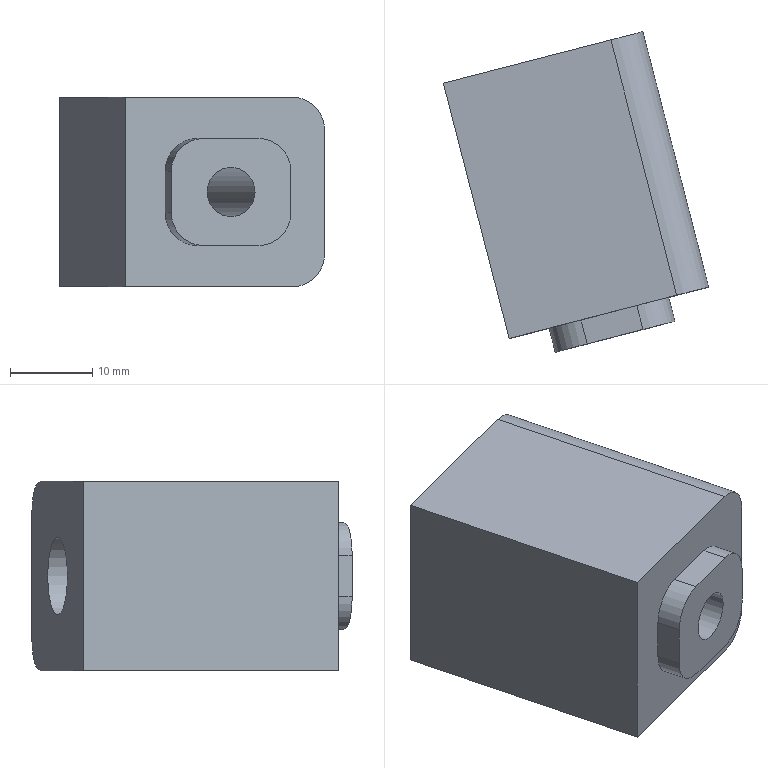Part | STEP file | 车灯-后视镜_id46_x_t | 1 solid | 20 faces | box 32.198 x 38.885 x 23 mm | volume 17479 mm3 | plane 12 | cylinder 8 | commonest cylinder face diameters 8 x6 6 x1 9.5 x1
STEP:
#1=CARTESIAN_POINT('',(-81.034,92.171,88.714));
#2=VERTEX_POINT('',#1);
#3=CARTESIAN_POINT('',(-81.034,92.171,103.714));
#4=VERTEX_POINT('',#3);
#5=CARTESIAN_POINT('',(-81.034,92.171,96.214));
#6=DIRECTION('',(0.,0.,1.));
#7=VECTOR('',#6,1.);
#8=LINE('',#5,#7);
#9=EDGE_CURVE('',#2,#4,#8,.T.);
#10=ORIENTED_EDGE('',*,*,#9,.T.);
#11=CARTESIAN_POINT('',(-84.907,91.172,107.714));
#12=VERTEX_POINT('',#11);
#13=CARTESIAN_POINT('',(-84.907,91.172,103.714));
#14=DIRECTION('',(0.2497,-0.9683,0.));
#15=DIRECTION('',(0.9683,0.2497,0.));
#16=AXIS2_PLACEMENT_3D('',#13,#14,#15);
#17=CIRCLE('',#16,4.);
#18=EDGE_CURVE('',#4,#12,#17,.T.);
#19=ORIENTED_EDGE('',*,*,#18,.T.);
#20=CARTESIAN_POINT('',(-105.242,85.928,107.714));
#21=VERTEX_POINT('',#20);
#22=CARTESIAN_POINT('',(-79.081,92.674,107.714));
#23=DIRECTION('',(-0.9683,-0.2497,0.));
#24=VECTOR('',#23,1.);
#25=LINE('',#22,#24);
#26=EDGE_CURVE('',#12,#21,#25,.T.);
#27=ORIENTED_EDGE('',*,*,#26,.T.);
#28=CARTESIAN_POINT('',(-105.242,85.928,84.714));
#29=VERTEX_POINT('',#28);
#30=CARTESIAN_POINT('',(-105.242,85.928,96.214));
#31=DIRECTION('',(0.,0.,1.));
#32=VECTOR('',#31,1.);
#33=LINE('',#30,#32);
#34=EDGE_CURVE('',#29,#21,#33,.T.);
#35=ORIENTED_EDGE('',*,*,#34,.F.);
#36=CARTESIAN_POINT('',(-84.907,91.172,84.714));
#37=VERTEX_POINT('',#36);
#38=CARTESIAN_POINT('',(-79.081,92.674,84.714));
#39=DIRECTION('',(0.9683,0.2497,0.));
#40=VECTOR('',#39,1.);
#41=LINE('',#38,#40);
#42=EDGE_CURVE('',#29,#37,#41,.T.);
#43=ORIENTED_EDGE('',*,*,#42,.T.);
#44=CARTESIAN_POINT('',(-84.907,91.172,88.714));
#45=DIRECTION('',(0.2497,-0.9683,0.));
#46=DIRECTION('',(0.9683,0.2497,0.));
#47=AXIS2_PLACEMENT_3D('',#44,#45,#46);
#48=CIRCLE('',#47,4.);
#49=EDGE_CURVE('',#37,#2,#48,.T.);
#50=ORIENTED_EDGE('',*,*,#49,.T.);
#51=EDGE_LOOP('',(#10,#19,#27,#35,#43,#50));
#52=FACE_BOUND('',#51,.T.);
#53=CARTESIAN_POINT('',(-89.749,89.923,89.714));
#54=VERTEX_POINT('',#53);
#55=CARTESIAN_POINT('',(-96.527,88.175,89.714));
#56=VERTEX_POINT('',#55);
#57=CARTESIAN_POINT('',(-105.242,85.928,89.714));
#58=DIRECTION('',(-0.9683,-0.2497,0.));
#59=VECTOR('',#58,1.);
#60=LINE('',#57,#59);
#61=EDGE_CURVE('',#54,#56,#60,.T.);
#62=ORIENTED_EDGE('',*,*,#61,.T.);
#63=CARTESIAN_POINT('',(-100.4,87.177,93.714));
#64=VERTEX_POINT('',#63);
#65=CARTESIAN_POINT('',(-96.527,88.175,93.714));
#66=DIRECTION('',(-0.2497,0.9683,0.));
#67=DIRECTION('',(0.9683,0.2497,0.));
#68=AXIS2_PLACEMENT_3D('',#65,#66,#67);
#69=CIRCLE('',#68,4.);
#70=EDGE_CURVE('',#56,#64,#69,.T.);
#71=ORIENTED_EDGE('',*,*,#70,.T.);
#72=CARTESIAN_POINT('',(-100.4,87.177,98.714));
#73=VERTEX_POINT('',#72);
#74=CARTESIAN_POINT('',(-100.4,87.177,107.714));
#75=DIRECTION('',(0.,0.,1.));
#76=VECTOR('',#75,1.);
#77=LINE('',#74,#76);
#78=EDGE_CURVE('',#64,#73,#77,.T.);
#79=ORIENTED_EDGE('',*,*,#78,.T.);
#80=CARTESIAN_POINT('',(-96.527,88.175,102.714));
#81=VERTEX_POINT('',#80);
#82=CARTESIAN_POINT('',(-96.527,88.175,98.714));
#83=DIRECTION('',(-0.2497,0.9683,0.));
#84=DIRECTION('',(0.9683,0.2497,0.));
#85=AXIS2_PLACEMENT_3D('',#82,#83,#84);
#86=CIRCLE('',#85,4.);
#87=EDGE_CURVE('',#73,#81,#86,.T.);
#88=ORIENTED_EDGE('',*,*,#87,.T.);
#89=CARTESIAN_POINT('',(-89.749,89.923,102.714));
#90=VERTEX_POINT('',#89);
#91=CARTESIAN_POINT('',(-105.242,85.928,102.714));
#92=DIRECTION('',(0.9683,0.2497,0.));
#93=VECTOR('',#92,1.);
#94=LINE('',#91,#93);
#95=EDGE_CURVE('',#81,#90,#94,.T.);
#96=ORIENTED_EDGE('',*,*,#95,.T.);
#97=CARTESIAN_POINT('',(-85.876,90.922,98.714));
#98=VERTEX_POINT('',#97);
#99=CARTESIAN_POINT('',(-89.749,89.923,98.714));
#100=DIRECTION('',(-0.2497,0.9683,0.));
#101=DIRECTION('',(0.9683,0.2497,0.));
#102=AXIS2_PLACEMENT_3D('',#99,#100,#101);
#103=CIRCLE('',#102,4.);
#104=EDGE_CURVE('',#90,#98,#103,.T.);
#105=ORIENTED_EDGE('',*,*,#104,.T.);
#106=CARTESIAN_POINT('',(-85.876,90.922,93.714));
#107=VERTEX_POINT('',#106);
#108=CARTESIAN_POINT('',(-85.876,90.922,107.714));
#109=DIRECTION('',(0.,0.,-1.));
#110=VECTOR('',#109,1.);
#111=LINE('',#108,#110);
#112=EDGE_CURVE('',#98,#107,#111,.T.);
#113=ORIENTED_EDGE('',*,*,#112,.T.);
#114=CARTESIAN_POINT('',(-89.749,89.923,93.714));
#115=DIRECTION('',(-0.2497,0.9683,0.));
#116=DIRECTION('',(0.9683,0.2497,0.));
#117=AXIS2_PLACEMENT_3D('',#114,#115,#116);
#118=CIRCLE('',#117,4.);
#119=EDGE_CURVE('',#107,#54,#118,.T.);
#120=ORIENTED_EDGE('',*,*,#119,.T.);
#121=EDGE_LOOP('',(#62,#71,#79,#88,#96,#105,#113,#120));
#122=FACE_BOUND('',#121,.T.);
#123=CARTESIAN_POINT('',(-105.242,85.928,96.214));
#124=DIRECTION('',(0.2497,-0.9683,0.));
#125=DIRECTION('',(0.9683,0.2497,0.));
#126=AXIS2_PLACEMENT_3D('',#123,#124,#125);
#127=PLANE('',#126);
#128=ADVANCED_FACE('',(#52,#122),#127,.T.);
#129=CARTESIAN_POINT('',(-113.232,116.914,84.714));
#130=VERTEX_POINT('',#129);
#131=CARTESIAN_POINT('',(-92.898,122.158,84.714));
#132=VERTEX_POINT('',#131);
#133=CARTESIAN_POINT('',(-87.071,123.66,84.714));
#134=DIRECTION('',(0.9683,0.2497,0.));
#135=VECTOR('',#134,1.);
#136=LINE('',#133,#135);
#137=EDGE_CURVE('',#130,#132,#136,.T.);
#138=ORIENTED_EDGE('',*,*,#137,.T.);
#139=CARTESIAN_POINT('',(-85.172,92.197,84.714));
#140=DIRECTION('',(0.2497,-0.9683,0.));
#141=VECTOR('',#140,1.);
#142=LINE('',#139,#141);
#143=EDGE_CURVE('',#132,#37,#142,.T.);
#144=ORIENTED_EDGE('',*,*,#143,.T.);
#145=ORIENTED_EDGE('',*,*,#42,.F.);
#146=CARTESIAN_POINT('',(-105.507,86.954,84.714));
#147=DIRECTION('',(-0.2497,0.9683,0.));
#148=VECTOR('',#147,1.);
#149=LINE('',#146,#148);
#150=EDGE_CURVE('',#29,#130,#149,.T.);
#151=ORIENTED_EDGE('',*,*,#150,.T.);
#152=EDGE_LOOP('',(#138,#144,#145,#151));
#153=FACE_OUTER_BOUND('',#152,.T.);
#154=CARTESIAN_POINT('',(-79.346,93.7,84.714));
#155=DIRECTION('',(0.,0.,1.));
#156=DIRECTION('',(-0.9764,-0.2158,0.));
#157=AXIS2_PLACEMENT_3D('',#154,#155,#156);
#158=PLANE('',#157);
#159=ADVANCED_FACE('',(#153),#158,.F.);
#160=ORIENTED_EDGE('',*,*,#26,.F.);
#161=CARTESIAN_POINT('',(-92.898,122.158,107.714));
#162=VERTEX_POINT('',#161);
#163=CARTESIAN_POINT('',(-85.172,92.197,107.714));
#164=DIRECTION('',(-0.2497,0.9683,0.));
#165=VECTOR('',#164,1.);
#166=LINE('',#163,#165);
#167=EDGE_CURVE('',#12,#162,#166,.T.);
#168=ORIENTED_EDGE('',*,*,#167,.T.);
#169=CARTESIAN_POINT('',(-113.232,116.914,107.714));
#170=VERTEX_POINT('',#169);
#171=CARTESIAN_POINT('',(-87.071,123.66,107.714));
#172=DIRECTION('',(-0.9683,-0.2497,0.));
#173=VECTOR('',#172,1.);
#174=LINE('',#171,#173);
#175=EDGE_CURVE('',#162,#170,#174,.T.);
#176=ORIENTED_EDGE('',*,*,#175,.T.);
#177=CARTESIAN_POINT('',(-102.312,74.565,107.714));
#178=DIRECTION('',(-0.2497,0.9683,0.));
#179=VECTOR('',#178,1.);
#180=LINE('',#177,#179);
#181=EDGE_CURVE('',#21,#170,#180,.T.);
#182=ORIENTED_EDGE('',*,*,#181,.F.);
#183=EDGE_LOOP('',(#160,#168,#176,#182));
#184=FACE_OUTER_BOUND('',#183,.T.);
#185=CARTESIAN_POINT('',(-79.346,93.7,107.714));
#186=DIRECTION('',(0.,0.,1.));
#187=DIRECTION('',(-0.9764,-0.2158,0.));
#188=AXIS2_PLACEMENT_3D('',#185,#186,#187);
#189=PLANE('',#188);
#190=ADVANCED_FACE('',(#184),#189,.T.);
#191=CARTESIAN_POINT('',(-89.024,123.157,88.714));
#192=VERTEX_POINT('',#191);
#193=CARTESIAN_POINT('',(-89.024,123.157,103.714));
#194=VERTEX_POINT('',#193);
#195=CARTESIAN_POINT('',(-89.024,123.157,96.214));
#196=DIRECTION('',(0.,0.,1.));
#197=VECTOR('',#196,1.);
#198=LINE('',#195,#197);
#199=EDGE_CURVE('',#192,#194,#198,.T.);
#200=ORIENTED_EDGE('',*,*,#199,.T.);
#201=CARTESIAN_POINT('',(-85.156,108.157,103.714));
#202=DIRECTION('',(0.2497,-0.9683,0.));
#203=VECTOR('',#202,1.);
#204=LINE('',#201,#203);
#205=EDGE_CURVE('',#194,#4,#204,.T.);
#206=ORIENTED_EDGE('',*,*,#205,.T.);
#207=ORIENTED_EDGE('',*,*,#9,.F.);
#208=CARTESIAN_POINT('',(-85.156,108.157,88.714));
#209=DIRECTION('',(-0.2497,0.9683,0.));
#210=VECTOR('',#209,1.);
#211=LINE('',#208,#210);
#212=EDGE_CURVE('',#2,#192,#211,.T.);
#213=ORIENTED_EDGE('',*,*,#212,.T.);
#214=EDGE_LOOP('',(#200,#206,#207,#213));
#215=FACE_OUTER_BOUND('',#214,.T.);
#216=CARTESIAN_POINT('',(-85.156,108.157,96.214));
#217=DIRECTION('',(-0.9683,-0.2497,0.));
#218=DIRECTION('',(0.2497,-0.9683,0.));
#219=AXIS2_PLACEMENT_3D('',#216,#217,#218);
#220=PLANE('',#219);
#221=ADVANCED_FACE('',(#215),#220,.F.);
#222=ORIENTED_EDGE('',*,*,#181,.T.);
#223=CARTESIAN_POINT('',(-113.232,116.914,-21.603));
#224=DIRECTION('',(0.,0.,-1.));
#225=VECTOR('',#224,1.);
#226=LINE('',#223,#225);
#227=EDGE_CURVE('',#170,#130,#226,.T.);
#228=ORIENTED_EDGE('',*,*,#227,.T.);
#229=ORIENTED_EDGE('',*,*,#150,.F.);
#230=ORIENTED_EDGE('',*,*,#34,.T.);
#231=EDGE_LOOP('',(#222,#228,#229,#230));
#232=FACE_OUTER_BOUND('',#231,.T.);
#233=CARTESIAN_POINT('',(-102.312,74.565,-21.603));
#234=DIRECTION('',(0.9683,0.2497,0.));
#235=DIRECTION('',(-0.2497,0.9683,0.));
#236=AXIS2_PLACEMENT_3D('',#233,#234,#235);
#237=PLANE('',#236);
#238=ADVANCED_FACE('',(#232),#237,.F.);
#239=CARTESIAN_POINT('',(-96.529,121.222,96.214));
#240=VERTEX_POINT('',#239);
#241=CARTESIAN_POINT('',(-101.128,120.036,96.214));
#242=DIRECTION('',(0.2497,-0.9683,0.));
#243=DIRECTION('',(0.9683,0.2497,0.));
#244=AXIS2_PLACEMENT_3D('',#241,#242,#243);
#245=CIRCLE('',#244,4.75);
#246=EDGE_CURVE('',#240,#240,#245,.T.);
#247=ORIENTED_EDGE('',*,*,#246,.T.);
#248=EDGE_LOOP('',(#247));
#249=FACE_BOUND('',#248,.T.);
#250=ORIENTED_EDGE('',*,*,#175,.F.);
#251=CARTESIAN_POINT('',(-92.898,122.158,103.714));
#252=DIRECTION('',(-0.2497,0.9683,0.));
#253=DIRECTION('',(0.9683,0.2497,0.));
#254=AXIS2_PLACEMENT_3D('',#251,#252,#253);
#255=CIRCLE('',#254,4.);
#256=EDGE_CURVE('',#162,#194,#255,.T.);
#257=ORIENTED_EDGE('',*,*,#256,.T.);
#258=ORIENTED_EDGE('',*,*,#199,.F.);
#259=CARTESIAN_POINT('',(-92.898,122.158,88.714));
#260=DIRECTION('',(-0.2497,0.9683,0.));
#261=DIRECTION('',(0.9683,0.2497,0.));
#262=AXIS2_PLACEMENT_3D('',#259,#260,#261);
#263=CIRCLE('',#262,4.);
#264=EDGE_CURVE('',#192,#132,#263,.T.);
#265=ORIENTED_EDGE('',*,*,#264,.T.);
#266=ORIENTED_EDGE('',*,*,#137,.F.);
#267=ORIENTED_EDGE('',*,*,#227,.F.);
#268=EDGE_LOOP('',(#250,#257,#258,#265,#266,#267));
#269=FACE_BOUND('',#268,.T.);
#270=CARTESIAN_POINT('',(-101.29,119.994,96.214));
#271=DIRECTION('',(0.2497,-0.9683,0.));
#272=DIRECTION('',(0.9683,0.2497,0.));
#273=AXIS2_PLACEMENT_3D('',#270,#271,#272);
#274=PLANE('',#273);
#275=ADVANCED_FACE('',(#249,#269),#274,.F.);
#276=CARTESIAN_POINT('',(-95.294,85.395,96.214));
#277=VERTEX_POINT('',#276);
#278=CARTESIAN_POINT('',(-92.389,86.144,96.214));
#279=DIRECTION('',(-0.2497,0.9683,0.));
#280=DIRECTION('',(-0.9683,-0.2497,0.));
#281=AXIS2_PLACEMENT_3D('',#278,#279,#280);
#282=CIRCLE('',#281,3.);
#283=EDGE_CURVE('',#277,#277,#282,.T.);
#284=ORIENTED_EDGE('',*,*,#283,.T.);
#285=EDGE_LOOP('',(#284));
#286=FACE_BOUND('',#285,.T.);
#287=CARTESIAN_POINT('',(-99.651,84.272,98.714));
#288=VERTEX_POINT('',#287);
#289=CARTESIAN_POINT('',(-99.651,84.272,93.714));
#290=VERTEX_POINT('',#289);
#291=CARTESIAN_POINT('',(-99.651,84.272,-21.603));
#292=DIRECTION('',(0.,0.,-1.));
#293=VECTOR('',#292,1.);
#294=LINE('',#291,#293);
#295=EDGE_CURVE('',#288,#290,#294,.T.);
#296=ORIENTED_EDGE('',*,*,#295,.T.);
#297=CARTESIAN_POINT('',(-95.778,85.27,89.714));
#298=VERTEX_POINT('',#297);
#299=CARTESIAN_POINT('',(-95.778,85.27,93.714));
#300=DIRECTION('',(0.2497,-0.9683,0.));
#301=DIRECTION('',(0.9683,0.2497,0.));
#302=AXIS2_PLACEMENT_3D('',#299,#300,#301);
#303=CIRCLE('',#302,4.);
#304=EDGE_CURVE('',#290,#298,#303,.T.);
#305=ORIENTED_EDGE('',*,*,#304,.T.);
#306=CARTESIAN_POINT('',(-89.,87.018,89.714));
#307=VERTEX_POINT('',#306);
#308=CARTESIAN_POINT('',(-78.332,89.769,89.714));
#309=DIRECTION('',(0.9683,0.2497,0.));
#310=VECTOR('',#309,1.);
#311=LINE('',#308,#310);
#312=EDGE_CURVE('',#298,#307,#311,.T.);
#313=ORIENTED_EDGE('',*,*,#312,.T.);
#314=CARTESIAN_POINT('',(-85.127,88.017,93.714));
#315=VERTEX_POINT('',#314);
#316=CARTESIAN_POINT('',(-89.,87.018,93.714));
#317=DIRECTION('',(0.2497,-0.9683,0.));
#318=DIRECTION('',(0.9683,0.2497,0.));
#319=AXIS2_PLACEMENT_3D('',#316,#317,#318);
#320=CIRCLE('',#319,4.);
#321=EDGE_CURVE('',#307,#315,#320,.T.);
#322=ORIENTED_EDGE('',*,*,#321,.T.);
#323=CARTESIAN_POINT('',(-85.127,88.017,98.714));
#324=VERTEX_POINT('',#323);
#325=CARTESIAN_POINT('',(-85.127,88.017,96.214));
#326=DIRECTION('',(0.,0.,1.));
#327=VECTOR('',#326,1.);
#328=LINE('',#325,#327);
#329=EDGE_CURVE('',#315,#324,#328,.T.);
#330=ORIENTED_EDGE('',*,*,#329,.T.);
#331=CARTESIAN_POINT('',(-89.,87.018,102.714));
#332=VERTEX_POINT('',#331);
#333=CARTESIAN_POINT('',(-89.,87.018,98.714));
#334=DIRECTION('',(0.2497,-0.9683,0.));
#335=DIRECTION('',(0.9683,0.2497,0.));
#336=AXIS2_PLACEMENT_3D('',#333,#334,#335);
#337=CIRCLE('',#336,4.);
#338=EDGE_CURVE('',#324,#332,#337,.T.);
#339=ORIENTED_EDGE('',*,*,#338,.T.);
#340=CARTESIAN_POINT('',(-95.778,85.27,102.714));
#341=VERTEX_POINT('',#340);
#342=CARTESIAN_POINT('',(-78.332,89.769,102.714));
#343=DIRECTION('',(-0.9683,-0.2497,0.));
#344=VECTOR('',#343,1.);
#345=LINE('',#342,#344);
#346=EDGE_CURVE('',#332,#341,#345,.T.);
#347=ORIENTED_EDGE('',*,*,#346,.T.);
#348=CARTESIAN_POINT('',(-95.778,85.27,98.714));
#349=DIRECTION('',(0.2497,-0.9683,0.));
#350=DIRECTION('',(0.9683,0.2497,0.));
#351=AXIS2_PLACEMENT_3D('',#348,#349,#350);
#352=CIRCLE('',#351,4.);
#353=EDGE_CURVE('',#341,#288,#352,.T.);
#354=ORIENTED_EDGE('',*,*,#353,.T.);
#355=EDGE_LOOP('',(#296,#305,#313,#322,#330,#339,#347,#354));
#356=FACE_BOUND('',#355,.T.);
#357=CARTESIAN_POINT('',(-92.389,86.144,96.214));
#358=DIRECTION('',(0.2497,-0.9683,0.));
#359=DIRECTION('',(0.9683,0.2497,0.));
#360=AXIS2_PLACEMENT_3D('',#357,#358,#359);
#361=PLANE('',#360);
#362=ADVANCED_FACE('',(#286,#356),#361,.T.);
#363=ORIENTED_EDGE('',*,*,#329,.F.);
#364=CARTESIAN_POINT('',(-89.998,106.908,93.714));
#365=DIRECTION('',(-0.2497,0.9683,0.));
#366=VECTOR('',#365,1.);
#367=LINE('',#364,#366);
#368=EDGE_CURVE('',#315,#107,#367,.T.);
#369=ORIENTED_EDGE('',*,*,#368,.T.);
#370=ORIENTED_EDGE('',*,*,#112,.F.);
#371=CARTESIAN_POINT('',(-89.998,106.908,98.714));
#372=DIRECTION('',(0.2497,-0.9683,0.));
#373=VECTOR('',#372,1.);
#374=LINE('',#371,#373);
#375=EDGE_CURVE('',#98,#324,#374,.T.);
#376=ORIENTED_EDGE('',*,*,#375,.T.);
#377=EDGE_LOOP('',(#363,#369,#370,#376));
#378=FACE_OUTER_BOUND('',#377,.T.);
#379=CARTESIAN_POINT('',(-89.998,106.908,96.214));
#380=DIRECTION('',(-0.9683,-0.2497,0.));
#381=DIRECTION('',(0.2497,-0.9683,0.));
#382=AXIS2_PLACEMENT_3D('',#379,#380,#381);
#383=PLANE('',#382);
#384=ADVANCED_FACE('',(#378),#383,.F.);
#385=ORIENTED_EDGE('',*,*,#346,.F.);
#386=CARTESIAN_POINT('',(-90.013,90.949,102.714));
#387=DIRECTION('',(-0.2497,0.9683,0.));
#388=VECTOR('',#387,1.);
#389=LINE('',#386,#388);
#390=EDGE_CURVE('',#332,#90,#389,.T.);
#391=ORIENTED_EDGE('',*,*,#390,.T.);
#392=ORIENTED_EDGE('',*,*,#95,.F.);
#393=CARTESIAN_POINT('',(-96.792,89.201,102.714));
#394=DIRECTION('',(0.2497,-0.9683,0.));
#395=VECTOR('',#394,1.);
#396=LINE('',#393,#395);
#397=EDGE_CURVE('',#81,#341,#396,.T.);
#398=ORIENTED_EDGE('',*,*,#397,.T.);
#399=EDGE_LOOP('',(#385,#391,#392,#398));
#400=FACE_OUTER_BOUND('',#399,.T.);
#401=CARTESIAN_POINT('',(-79.346,93.7,102.714));
#402=DIRECTION('',(0.,0.,1.));
#403=DIRECTION('',(-0.9764,-0.2158,0.));
#404=AXIS2_PLACEMENT_3D('',#401,#402,#403);
#405=PLANE('',#404);
#406=ADVANCED_FACE('',(#400),#405,.T.);
#407=ORIENTED_EDGE('',*,*,#78,.F.);
#408=CARTESIAN_POINT('',(-97.47,75.813,93.714));
#409=DIRECTION('',(0.2497,-0.9683,0.));
#410=VECTOR('',#409,1.);
#411=LINE('',#408,#410);
#412=EDGE_CURVE('',#64,#290,#411,.T.);
#413=ORIENTED_EDGE('',*,*,#412,.T.);
#414=ORIENTED_EDGE('',*,*,#295,.F.);
#415=CARTESIAN_POINT('',(-97.47,75.813,98.714));
#416=DIRECTION('',(-0.2497,0.9683,0.));
#417=VECTOR('',#416,1.);
#418=LINE('',#415,#417);
#419=EDGE_CURVE('',#288,#73,#418,.T.);
#420=ORIENTED_EDGE('',*,*,#419,.T.);
#421=EDGE_LOOP('',(#407,#413,#414,#420));
#422=FACE_OUTER_BOUND('',#421,.T.);
#423=CARTESIAN_POINT('',(-97.47,75.813,-21.603));
#424=DIRECTION('',(0.9683,0.2497,0.));
#425=DIRECTION('',(-0.2497,0.9683,0.));
#426=AXIS2_PLACEMENT_3D('',#423,#424,#425);
#427=PLANE('',#426);
#428=ADVANCED_FACE('',(#422),#427,.F.);
#429=ORIENTED_EDGE('',*,*,#312,.F.);
#430=CARTESIAN_POINT('',(-96.792,89.201,89.714));
#431=DIRECTION('',(-0.2497,0.9683,0.));
#432=VECTOR('',#431,1.);
#433=LINE('',#430,#432);
#434=EDGE_CURVE('',#298,#56,#433,.T.);
#435=ORIENTED_EDGE('',*,*,#434,.T.);
#436=ORIENTED_EDGE('',*,*,#61,.F.);
#437=CARTESIAN_POINT('',(-90.013,90.949,89.714));
#438=DIRECTION('',(0.2497,-0.9683,0.));
#439=VECTOR('',#438,1.);
#440=LINE('',#437,#439);
#441=EDGE_CURVE('',#54,#307,#440,.T.);
#442=ORIENTED_EDGE('',*,*,#441,.T.);
#443=EDGE_LOOP('',(#429,#435,#436,#442));
#444=FACE_OUTER_BOUND('',#443,.T.);
#445=CARTESIAN_POINT('',(-79.346,93.7,89.714));
#446=DIRECTION('',(0.,0.,1.));
#447=DIRECTION('',(-0.9764,-0.2158,0.));
#448=AXIS2_PLACEMENT_3D('',#445,#446,#447);
#449=PLANE('',#448);
#450=ADVANCED_FACE('',(#444),#449,.F.);
#451=ORIENTED_EDGE('',*,*,#104,.F.);
#452=ORIENTED_EDGE('',*,*,#390,.F.);
#453=ORIENTED_EDGE('',*,*,#338,.F.);
#454=ORIENTED_EDGE('',*,*,#375,.F.);
#455=EDGE_LOOP('',(#451,#452,#453,#454));
#456=FACE_OUTER_BOUND('',#455,.T.);
#457=CARTESIAN_POINT('',(-93.871,105.91,98.714));
#458=DIRECTION('',(-0.2497,0.9683,0.));
#459=DIRECTION('',(-0.9683,-0.2497,0.));
#460=AXIS2_PLACEMENT_3D('',#457,#458,#459);
#461=CYLINDRICAL_SURFACE('',#460,4.);
#462=ADVANCED_FACE('',(#456),#461,.T.);
#463=ORIENTED_EDGE('',*,*,#87,.F.);
#464=ORIENTED_EDGE('',*,*,#419,.F.);
#465=ORIENTED_EDGE('',*,*,#353,.F.);
#466=ORIENTED_EDGE('',*,*,#397,.F.);
#467=EDGE_LOOP('',(#463,#464,#465,#466));
#468=FACE_OUTER_BOUND('',#467,.T.);
#469=CARTESIAN_POINT('',(-96.792,89.201,98.714));
#470=DIRECTION('',(-0.2497,0.9683,0.));
#471=DIRECTION('',(-0.9683,-0.2497,0.));
#472=AXIS2_PLACEMENT_3D('',#469,#470,#471);
#473=CYLINDRICAL_SURFACE('',#472,4.);
#474=ADVANCED_FACE('',(#468),#473,.T.);
#475=ORIENTED_EDGE('',*,*,#70,.F.);
#476=ORIENTED_EDGE('',*,*,#434,.F.);
#477=ORIENTED_EDGE('',*,*,#304,.F.);
#478=ORIENTED_EDGE('',*,*,#412,.F.);
#479=EDGE_LOOP('',(#475,#476,#477,#478));
#480=FACE_OUTER_BOUND('',#479,.T.);
#481=CARTESIAN_POINT('',(-93.597,76.812,93.714));
#482=DIRECTION('',(0.2497,-0.9683,0.));
#483=DIRECTION('',(0.9683,0.2497,0.));
#484=AXIS2_PLACEMENT_3D('',#481,#482,#483);
#485=CYLINDRICAL_SURFACE('',#484,4.);
#486=ADVANCED_FACE('',(#480),#485,.T.);
#487=ORIENTED_EDGE('',*,*,#119,.F.);
#488=ORIENTED_EDGE('',*,*,#368,.F.);
#489=ORIENTED_EDGE('',*,*,#321,.F.);
#490=ORIENTED_EDGE('',*,*,#441,.F.);
#491=EDGE_LOOP('',(#487,#488,#489,#490));
#492=FACE_OUTER_BOUND('',#491,.T.);
#493=CARTESIAN_POINT('',(-90.013,90.949,93.714));
#494=DIRECTION('',(0.2497,-0.9683,0.));
#495=DIRECTION('',(0.9683,0.2497,0.));
#496=AXIS2_PLACEMENT_3D('',#493,#494,#495);
#497=CYLINDRICAL_SURFACE('',#496,4.);
#498=ADVANCED_FACE('',(#492),#497,.T.);
#499=CARTESIAN_POINT('',(-96.725,114.975,96.214));
#500=VERTEX_POINT('',#499);
#501=CARTESIAN_POINT('',(-99.63,114.226,96.214));
#502=DIRECTION('',(-0.2497,0.9683,0.));
#503=DIRECTION('',(0.9683,0.2497,0.));
#504=AXIS2_PLACEMENT_3D('',#501,#502,#503);
#505=CIRCLE('',#504,3.);
#506=EDGE_CURVE('',#500,#500,#505,.T.);
#507=ORIENTED_EDGE('',*,*,#506,.T.);
#508=EDGE_LOOP('',(#507));
#509=FACE_BOUND('',#508,.T.);
#510=ORIENTED_EDGE('',*,*,#283,.F.);
#511=EDGE_LOOP('',(#510));
#512=FACE_BOUND('',#511,.T.);
#513=CARTESIAN_POINT('',(-92.389,86.144,96.214));
#514=DIRECTION('',(-0.2497,0.9683,0.));
#515=DIRECTION('',(-0.9683,-0.2497,0.));
#516=AXIS2_PLACEMENT_3D('',#513,#514,#515);
#517=CYLINDRICAL_SURFACE('',#516,3.);
#518=ADVANCED_FACE('',(#509,#512),#517,.F.);
#519=ORIENTED_EDGE('',*,*,#506,.F.);
#520=EDGE_LOOP('',(#519));
#521=FACE_BOUND('',#520,.T.);
#522=CARTESIAN_POINT('',(-104.23,113.04,96.214));
#523=VERTEX_POINT('',#522);
#524=CARTESIAN_POINT('',(-99.63,114.226,96.214));
#525=DIRECTION('',(-0.2497,0.9683,0.));
#526=DIRECTION('',(-0.9683,-0.2497,0.));
#527=AXIS2_PLACEMENT_3D('',#524,#525,#526);
#528=CIRCLE('',#527,4.75);
#529=EDGE_CURVE('',#523,#523,#528,.T.);
#530=ORIENTED_EDGE('',*,*,#529,.T.);
#531=EDGE_LOOP('',(#530));
#532=FACE_BOUND('',#531,.T.);
#533=CARTESIAN_POINT('',(-99.63,114.226,96.214));
#534=DIRECTION('',(0.2497,-0.9683,0.));
#535=DIRECTION('',(0.9683,0.2497,0.));
#536=AXIS2_PLACEMENT_3D('',#533,#534,#535);
#537=PLANE('',#536);
#538=ADVANCED_FACE('',(#521,#532),#537,.F.);
#539=ORIENTED_EDGE('',*,*,#529,.F.);
#540=EDGE_LOOP('',(#539));
#541=FACE_BOUND('',#540,.T.);
#542=ORIENTED_EDGE('',*,*,#246,.F.);
#543=EDGE_LOOP('',(#542));
#544=FACE_BOUND('',#543,.T.);
#545=CARTESIAN_POINT('',(-101.128,120.036,96.214));
#546=DIRECTION('',(0.2497,-0.9683,0.));
#547=DIRECTION('',(0.9683,0.2497,0.));
#548=AXIS2_PLACEMENT_3D('',#545,#546,#547);
#549=CYLINDRICAL_SURFACE('',#548,4.75);
#550=ADVANCED_FACE('',(#541,#544),#549,.F.);
#551=ORIENTED_EDGE('',*,*,#18,.F.);
#552=ORIENTED_EDGE('',*,*,#205,.F.);
#553=ORIENTED_EDGE('',*,*,#256,.F.);
#554=ORIENTED_EDGE('',*,*,#167,.F.);
#555=EDGE_LOOP('',(#551,#552,#553,#554));
#556=FACE_OUTER_BOUND('',#555,.T.);
#557=CARTESIAN_POINT('',(-85.172,92.197,103.714));
#558=DIRECTION('',(0.2497,-0.9683,0.));
#559=DIRECTION('',(0.9683,0.2497,0.));
#560=AXIS2_PLACEMENT_3D('',#557,#558,#559);
#561=CYLINDRICAL_SURFACE('',#560,4.);
#562=ADVANCED_FACE('',(#556),#561,.T.);
#563=ORIENTED_EDGE('',*,*,#264,.F.);
#564=ORIENTED_EDGE('',*,*,#212,.F.);
#565=ORIENTED_EDGE('',*,*,#49,.F.);
#566=ORIENTED_EDGE('',*,*,#143,.F.);
#567=EDGE_LOOP('',(#563,#564,#565,#566));
#568=FACE_OUTER_BOUND('',#567,.T.);
#569=CARTESIAN_POINT('',(-85.172,92.197,88.714));
#570=DIRECTION('',(0.2497,-0.9683,0.));
#571=DIRECTION('',(0.9683,0.2497,0.));
#572=AXIS2_PLACEMENT_3D('',#569,#570,#571);
#573=CYLINDRICAL_SURFACE('',#572,4.);
#574=ADVANCED_FACE('',(#568),#573,.T.);
#575=CLOSED_SHELL('',(#128,#159,#190,#221,#238,#275,#362,#384,#406,#428,#450,#462,#474,#486,#498,#518,#538,#550,#562,#574));
#576=MANIFOLD_SOLID_BREP('',#575);
#577=(LENGTH_UNIT()NAMED_UNIT(*)SI_UNIT(.MILLI.,.METRE.));
#578=UNCERTAINTY_MEASURE_WITH_UNIT(LENGTH_MEASURE(0.00002),#577,'','');
#579=(NAMED_UNIT(*)PLANE_ANGLE_UNIT()SI_UNIT($,.RADIAN.));
#580=PLANE_ANGLE_MEASURE_WITH_UNIT(PLANE_ANGLE_MEASURE(0.01745),#579);
#581=DIMENSIONAL_EXPONENTS(0.,0.,0.,0.,0.,0.,0.);
#582=(CONVERSION_BASED_UNIT('DEGREE',#580)NAMED_UNIT(#581)PLANE_ANGLE_UNIT());
#583=(NAMED_UNIT(*)SI_UNIT($,.STERADIAN.)SOLID_ANGLE_UNIT());
#584=(GEOMETRIC_REPRESENTATION_CONTEXT(3)GLOBAL_UNCERTAINTY_ASSIGNED_CONTEXT((#578))GLOBAL_UNIT_ASSIGNED_CONTEXT((#577,#582,#583))REPRESENTATION_CONTEXT('',''));
#585=ADVANCED_BREP_SHAPE_REPRESENTATION('',(#576),#584);